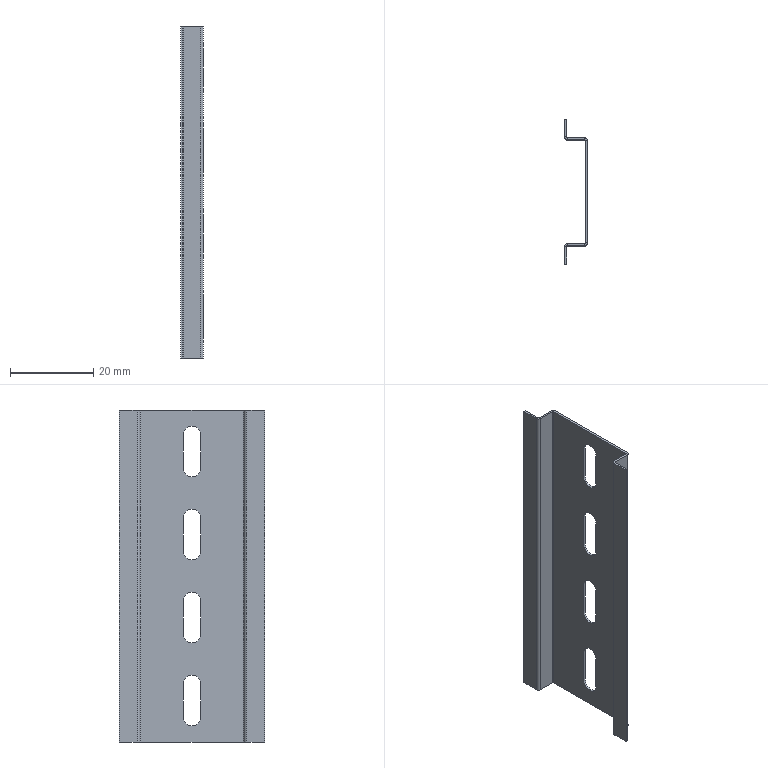Part | STEP file | DIN rail L60 | 1 solid | 54 faces | box 5.5 x 35 x 80 mm | volume 1674 mm3 | plane 38 | cylinder 16 | commonest cylinder face diameters 4.2 x8 0.4 x4 1.4 x4